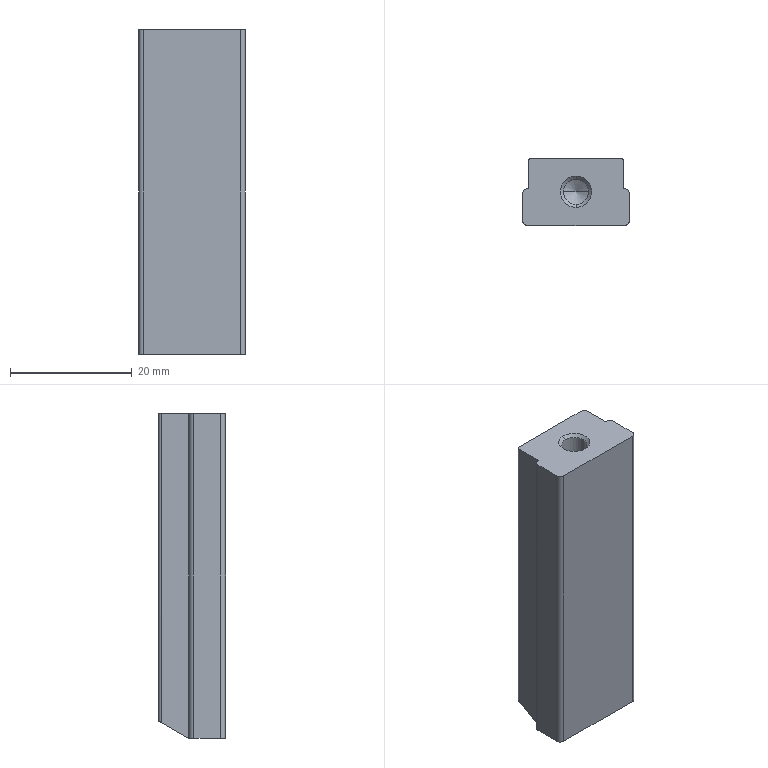Part | STEP file | LUOI GA PHIA TREN | 1 solid | 23 faces | box 17.5 x 11 x 53.3 mm | volume 9330 mm3 | plane 11 | cylinder 8 | cone 4 | commonest cylinder face diameters 1.6 x4 1 x2 4.134 x2